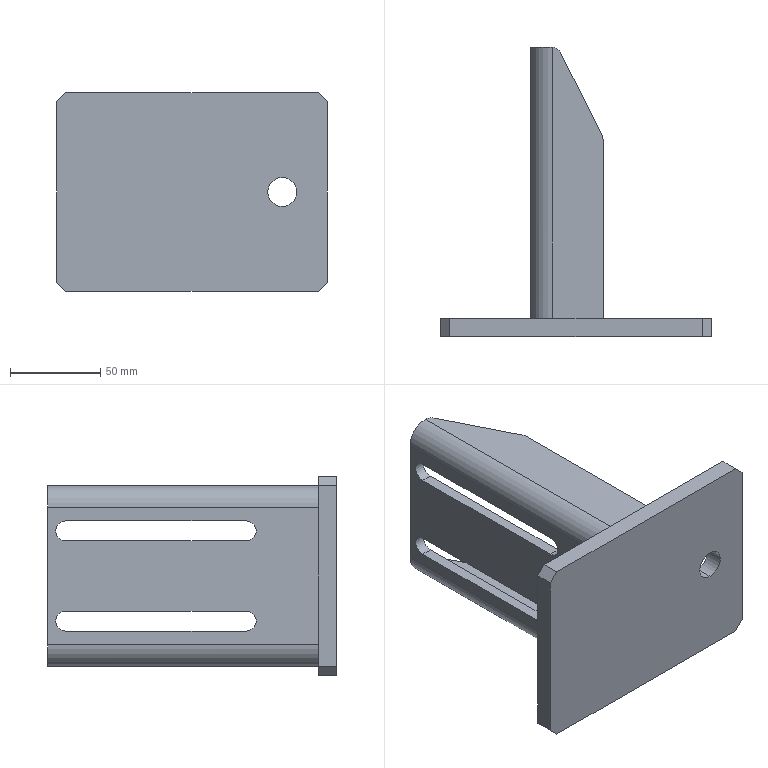Part | STEP file | PN_0031_foot mounting_default_machined_ | 2 solids | 40 faces | box 150 x 160 x 110 mm | volume 284875 mm3 | plane 26 | cylinder 14 | commonest cylinder face diameters 10 x4 11 x4 12 x2 16 x2 24 x2